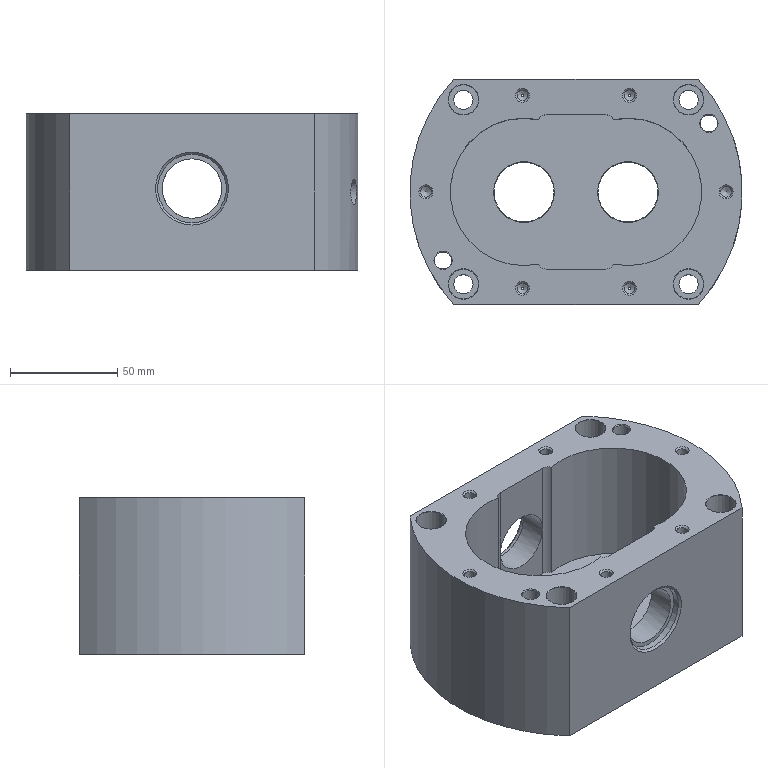NC program | NX | posted with a generic post | part box 155 x 105 x 73.2 mm
Lines 466 to 1316 of 30727:
(FLOOR_WALL_1_1 , TOOL : D25R0.5)
N912 T05 M6
N914 G54
N916 G17 G0 G90 X7.943 Y5.142 B0. C0. S2000 M3
N918 G43 Z30. H5
N920 Z1.5
N922 G94 G1 X6.744 Y5.554 Z1.467 F1000.
N924 X6.026 Y5.85 Z1.446
N926 X-6.026 Z1.131
N928 X-6.744 Y5.554 Z1.111
N930 X-8.656 Y4.897 Z1.058
N932 X-10.608 Y4.369 Z1.005
N934 X-12.591 Y3.974 Z0.952
N936 X-14.595 Y3.711 Z0.899
N938 X-16.613 Y3.584 Z0.846
N940 X-18.635 Y3.593 Z0.793
N942 X-20.652 Y3.736 Z0.74
N944 X-22.655 Y4.015 Z0.687
N946 X-23.416 Y4.167 Z0.667
N948 X-23.702 Y4.225 Z0.659
N950 X-24.464 Y4.255 Z0.639
N952 X-25.219 Y4.148 Z0.619
N954 X-25.943 Y3.909 Z0.599
N956 X-26.613 Y3.545 Z0.579
N958 X-27.207 Y3.067 Z0.559
N960 X-27.706 Y2.491 Z0.539
N962 X-28.095 Y1.835 Z0.519
N964 X-28.36 Y1.12 Z0.499
N966 X-28.475 Y0.548 Z0.484
N968 X-28.505 Y-0.214 Z0.464
N970 X-28.398 Y-0.969 Z0.444
N972 X-28.159 Y-1.693 Z0.424
N974 X-27.795 Y-2.363 Z0.404
N976 X-27.317 Y-2.957 Z0.384
N978 X-26.741 Y-3.456 Z0.364
N980 X-26.085 Y-3.845 Z0.344
N982 X-25.37 Y-4.11 Z0.324
N984 X-25.084 Y-4.167 Z0.317
N986 X-24.798 Y-4.225 Z0.309
N988 X-24.25 Y-4.26 Z0.295
N990 X-23.702 Y-4.225 Z0.28
N992 X-22.655 Y-4.015 Z0.252
N994 X-20.652 Y-3.736 Z0.199
N996 X-18.635 Y-3.593 Z0.146
N998 X-16.613 Y-3.584 Z0.093
N1000 X-14.595 Y-3.711 Z0.04
N1002 X-12.591 Y-3.974 Z-0.012
N1004 X-10.608 Y-4.369 Z-0.065
N1006 X-8.656 Y-4.897 Z-0.118
N1008 X-6.744 Y-5.554 Z-0.171
N1010 X-6.026 Y-5.85 Z-0.192
N1012 X0. Z-0.349
N1014 X6.026 F2200.
N1016 G2 X23.416 Y-4.167 R30.15
N1018 G3 X23.416 Y4.167 R-4.25
N1020 G2 X6.026 Y5.85 R30.15
N1022 G1 X-6.026
N1024 G2 X-23.416 Y4.167 R30.15
N1026 G3 X-23.416 Y-4.167 R-4.25
N1028 G2 X-6.026 Y-5.85 R30.15
N1030 G1 X0.
N1032 Y-23.35
N1034 X10.271
N1036 G2 X19.982 Y-21.327 R12.65
N1038 G3 X19.982 Y21.327 R-21.75
N1040 G2 X10.271 Y23.35 R12.65
N1042 G1 X-10.271
N1044 G2 X-19.982 Y21.327 R12.65
N1046 G3 X-19.982 Y-21.327 R-21.75
N1048 G2 X-10.271 Y-23.35 R12.65
N1050 G1 X0.
N1052 Z1.151
N1054 G0 X7.943 Y5.142
N1056 G1 X6.744 Y5.554 Z1.117 F1000.
N1058 X6.026 Y5.85 Z1.097
N1060 X-6.026 Z0.781
N1062 X-6.744 Y5.554 Z0.761
N1064 X-8.656 Y4.897 Z0.708
N1066 X-10.608 Y4.369 Z0.655
N1068 X-12.591 Y3.974 Z0.602
N1070 X-14.595 Y3.711 Z0.549
N1072 X-16.613 Y3.584 Z0.496
N1074 X-18.635 Y3.593 Z0.443
N1076 X-20.652 Y3.736 Z0.39
N1078 X-22.655 Y4.015 Z0.338
N1080 X-23.416 Y4.167 Z0.317
N1082 X-23.702 Y4.225 Z0.31
N1084 X-24.464 Y4.255 Z0.29
N1086 X-25.219 Y4.148 Z0.27
N1088 X-25.943 Y3.909 Z0.25
N1090 X-26.613 Y3.545 Z0.23
N1092 X-27.207 Y3.067 Z0.21
N1094 X-27.706 Y2.491 Z0.19
N1096 X-28.095 Y1.835 Z0.17
N1098 X-28.36 Y1.12 Z0.15
N1100 X-28.475 Y0.548 Z0.135
N1102 X-28.505 Y-0.214 Z0.115
N1104 X-28.398 Y-0.969 Z0.095
N1106 X-28.159 Y-1.693 Z0.075
N1108 X-27.795 Y-2.363 Z0.055
N1110 X-27.317 Y-2.957 Z0.035
N1112 X-26.741 Y-3.456 Z0.015
N1114 X-26.085 Y-3.845 Z-0.005
N1116 X-25.37 Y-4.11 Z-0.025
N1118 X-25.084 Y-4.167 Z-0.033
N1120 X-24.798 Y-4.225 Z-0.04
N1122 X-24.25 Y-4.26 Z-0.055
N1124 X-23.702 Y-4.225 Z-0.069
N1126 X-22.655 Y-4.015 Z-0.097
N1128 X-20.652 Y-3.736 Z-0.15
N1130 X-18.635 Y-3.593 Z-0.203
N1132 X-16.613 Y-3.584 Z-0.256
N1134 X-14.595 Y-3.711 Z-0.309
N1136 X-12.591 Y-3.974 Z-0.362
N1138 X-10.608 Y-4.369 Z-0.415
N1140 X-8.656 Y-4.897 Z-0.468
N1142 X-6.744 Y-5.554 Z-0.521
N1144 X-6.026 Y-5.85 Z-0.541
N1146 X0. Z-0.699
N1148 X6.026 F2200.
N1150 G2 X23.416 Y-4.167 R30.15
N1152 G3 X23.416 Y4.167 R-4.25
N1154 G2 X6.026 Y5.85 R30.15
N1156 G1 X-6.026
N1158 G2 X-23.416 Y4.167 R30.15
N1160 G3 X-23.416 Y-4.167 R-4.25
N1162 G2 X-6.026 Y-5.85 R30.15
N1164 G1 X0.
N1166 Y-23.35
N1168 X10.271
N1170 G2 X19.982 Y-21.327 R12.65
N1172 G3 X19.982 Y21.327 R-21.75
N1174 G2 X10.271 Y23.35 R12.65
N1176 G1 X-10.271
N1178 G2 X-19.982 Y21.327 R12.65
N1180 G3 X-19.982 Y-21.327 R-21.75
N1182 G2 X-10.271 Y-23.35 R12.65
N1184 G1 X0.
N1186 Z0.801
N1188 G0 X7.943 Y5.142
N1190 G1 X6.744 Y5.554 Z0.768 F1000.
N1192 X6.026 Y5.85 Z0.748
N1194 X-6.026 Z0.432
N1196 X-6.744 Y5.554 Z0.412
N1198 X-8.656 Y4.897 Z0.359
N1200 X-10.608 Y4.369 Z0.306
N1202 X-12.591 Y3.974 Z0.253
N1204 X-14.595 Y3.711 Z0.2
N1206 X-16.613 Y3.584 Z0.147
N1208 X-18.635 Y3.593 Z0.094
N1210 X-20.652 Y3.736 Z0.041
N1212 X-22.655 Y4.015 Z-0.012
N1214 X-23.416 Y4.167 Z-0.032
N1216 X-23.702 Y4.225 Z-0.04
N1218 X-24.464 Y4.255 Z-0.06
N1220 X-25.219 Y4.148 Z-0.08
N1222 X-25.943 Y3.909 Z-0.1
N1224 X-26.613 Y3.545 Z-0.12
N1226 X-27.207 Y3.067 Z-0.14
N1228 X-27.706 Y2.491 Z-0.16
N1230 X-28.095 Y1.835 Z-0.18
N1232 X-28.36 Y1.12 Z-0.2
N1234 X-28.475 Y0.548 Z-0.215
N1236 X-28.505 Y-0.214 Z-0.235
N1238 X-28.398 Y-0.969 Z-0.255
N1240 X-28.159 Y-1.693 Z-0.275
N1242 X-27.795 Y-2.363 Z-0.295
N1244 X-27.317 Y-2.957 Z-0.315
N1246 X-26.741 Y-3.456 Z-0.335
N1248 X-26.085 Y-3.845 Z-0.355
N1250 X-25.37 Y-4.11 Z-0.375
N1252 X-25.084 Y-4.167 Z-0.382
N1254 X-24.798 Y-4.225 Z-0.39
N1256 X-24.25 Y-4.26 Z-0.404
N1258 X-23.702 Y-4.225 Z-0.419
N1260 X-22.655 Y-4.015 Z-0.447
N1262 X-20.652 Y-3.736 Z-0.5
N1264 X-18.635 Y-3.593 Z-0.552
N1266 X-16.613 Y-3.584 Z-0.605
N1268 X-14.595 Y-3.711 Z-0.658
N1270 X-12.591 Y-3.974 Z-0.711
N1272 X-10.608 Y-4.369 Z-0.764
N1274 X-8.656 Y-4.897 Z-0.817
N1276 X-6.744 Y-5.554 Z-0.87
N1278 X-6.026 Y-5.85 Z-0.89
N1280 X0. Z-1.048
N1282 X6.026 F2200.
N1284 G2 X23.416 Y-4.167 R30.15
N1286 G3 X23.416 Y4.167 R-4.25
N1288 G2 X6.026 Y5.85 R30.15
N1290 G1 X-6.026
N1292 G2 X-23.416 Y4.167 R30.15
N1294 G3 X-23.416 Y-4.167 R-4.25
N1296 G2 X-6.026 Y-5.85 R30.15
N1298 G1 X0.
N1300 Y-23.35
N1302 X10.271
N1304 G2 X19.982 Y-21.327 R12.65
N1306 G3 X19.982 Y21.327 R-21.75
N1308 G2 X10.271 Y23.35 R12.65
N1310 G1 X-10.271
N1312 G2 X-19.982 Y21.327 R12.65
N1314 G3 X-19.982 Y-21.327 R-21.75
N1316 G2 X-10.271 Y-23.35 R12.65
N1318 G1 X0.
N1320 Z0.452
N1322 G0 X7.943 Y5.142
N1324 G1 X6.744 Y5.554 Z0.419 F1000.
N1326 X6.026 Y5.85 Z0.398
N1328 X-6.026 Z0.083
N1330 X-6.744 Y5.554 Z0.062
N1332 X-8.656 Y4.897 Z0.009
N1334 X-10.608 Y4.369 Z-0.044
N1336 X-12.591 Y3.974 Z-0.097
N1338 X-14.595 Y3.711 Z-0.15
N1340 X-16.613 Y3.584 Z-0.202
N1342 X-18.635 Y3.593 Z-0.255
N1344 X-20.652 Y3.736 Z-0.308
N1346 X-22.655 Y4.015 Z-0.361
N1348 X-23.416 Y4.167 Z-0.382
N1350 X-23.702 Y4.225 Z-0.389
N1352 X-24.464 Y4.255 Z-0.409
N1354 X-25.219 Y4.148 Z-0.429
N1356 X-25.943 Y3.909 Z-0.449
N1358 X-26.613 Y3.545 Z-0.469
N1360 X-27.207 Y3.067 Z-0.489
N1362 X-27.706 Y2.491 Z-0.509
N1364 X-28.095 Y1.835 Z-0.529
N1366 X-28.36 Y1.12 Z-0.549
N1368 X-28.475 Y0.548 Z-0.564
N1370 X-28.505 Y-0.214 Z-0.584
N1372 X-28.398 Y-0.969 Z-0.604
N1374 X-28.159 Y-1.693 Z-0.624
N1376 X-27.795 Y-2.363 Z-0.644
N1378 X-27.317 Y-2.957 Z-0.664
N1380 X-26.741 Y-3.456 Z-0.684
N1382 X-26.085 Y-3.845 Z-0.704
N1384 X-25.37 Y-4.11 Z-0.724
N1386 X-25.084 Y-4.167 Z-0.732
N1388 X-24.798 Y-4.225 Z-0.739
N1390 X-24.25 Y-4.26 Z-0.754
N1392 X-23.702 Y-4.225 Z-0.768
N1394 X-22.655 Y-4.015 Z-0.796
N1396 X-20.652 Y-3.736 Z-0.849
N1398 X-18.635 Y-3.593 Z-0.902
N1400 X-16.613 Y-3.584 Z-0.955
N1402 X-14.595 Y-3.711 Z-1.008
N1404 X-12.591 Y-3.974 Z-1.061
N1406 X-10.608 Y-4.369 Z-1.114
N1408 X-8.656 Y-4.897 Z-1.167
N1410 X-6.744 Y-5.554 Z-1.22
N1412 X-6.026 Y-5.85 Z-1.24
N1414 X0. Z-1.398
N1416 X6.026 F2200.
N1418 G2 X23.416 Y-4.167 R30.15
N1420 G3 X23.416 Y4.167 R-4.25
N1422 G2 X6.026 Y5.85 R30.15
N1424 G1 X-6.026
N1426 G2 X-23.416 Y4.167 R30.15
N1428 G3 X-23.416 Y-4.167 R-4.25
N1430 G2 X-6.026 Y-5.85 R30.15
N1432 G1 X0.
N1434 Y-23.35
N1436 X10.271
N1438 G2 X19.982 Y-21.327 R12.65
N1440 G3 X19.982 Y21.327 R-21.75
N1442 G2 X10.271 Y23.35 R12.65
N1444 G1 X-10.271
N1446 G2 X-19.982 Y21.327 R12.65
N1448 G3 X-19.982 Y-21.327 R-21.75
N1450 G2 X-10.271 Y-23.35 R12.65
N1452 G1 X0.
N1454 Z0.102
N1456 G0 X7.943 Y5.142
N1458 G1 X6.744 Y5.554 Z0.069 F1000.
N1460 X6.026 Y5.85 Z0.049
N1462 X-6.026 Z-0.267
N1464 X-6.744 Y5.554 Z-0.287
N1466 X-8.656 Y4.897 Z-0.34
N1468 X-10.608 Y4.369 Z-0.393
N1470 X-12.591 Y3.974 Z-0.446
N1472 X-14.595 Y3.711 Z-0.499
N1474 X-16.613 Y3.584 Z-0.552
N1476 X-18.635 Y3.593 Z-0.605
N1478 X-20.652 Y3.736 Z-0.658
N1480 X-22.655 Y4.015 Z-0.711
N1482 X-23.416 Y4.167 Z-0.731
N1484 X-23.702 Y4.225 Z-0.739
N1486 X-24.464 Y4.255 Z-0.759
N1488 X-25.219 Y4.148 Z-0.779
N1490 X-25.943 Y3.909 Z-0.799
N1492 X-26.613 Y3.545 Z-0.819
N1494 X-27.207 Y3.067 Z-0.839
N1496 X-27.706 Y2.491 Z-0.858
N1498 X-28.095 Y1.835 Z-0.878
N1500 X-28.36 Y1.12 Z-0.898
N1502 X-28.475 Y0.548 Z-0.914
N1504 X-28.505 Y-0.214 Z-0.934
N1506 X-28.398 Y-0.969 Z-0.954
N1508 X-28.159 Y-1.693 Z-0.974
N1510 X-27.795 Y-2.363 Z-0.994
N1512 X-27.317 Y-2.957 Z-1.014
N1514 X-26.741 Y-3.456 Z-1.033
N1516 X-26.085 Y-3.845 Z-1.053
N1518 X-25.37 Y-4.11 Z-1.073
N1520 X-25.084 Y-4.167 Z-1.081
N1522 X-24.798 Y-4.225 Z-1.089
N1524 X-24.25 Y-4.26 Z-1.103
N1526 X-23.702 Y-4.225 Z-1.117
N1528 X-22.655 Y-4.015 Z-1.145
N1530 X-20.652 Y-3.736 Z-1.198
N1532 X-18.635 Y-3.593 Z-1.251
N1534 X-16.613 Y-3.584 Z-1.304
N1536 X-14.595 Y-3.711 Z-1.357
N1538 X-12.591 Y-3.974 Z-1.41
N1540 X-10.608 Y-4.369 Z-1.463
N1542 X-8.656 Y-4.897 Z-1.516
N1544 X-6.744 Y-5.554 Z-1.569
N1546 X-6.026 Y-5.85 Z-1.589
N1548 X0. Z-1.747
N1550 X6.026 F2200.
N1552 G2 X23.416 Y-4.167 R30.15
N1554 G3 X23.416 Y4.167 R-4.25
N1556 G2 X6.026 Y5.85 R30.15
N1558 G1 X-6.026
N1560 G2 X-23.416 Y4.167 R30.15
N1562 G3 X-23.416 Y-4.167 R-4.25
N1564 G2 X-6.026 Y-5.85 R30.15
N1566 G1 X0.
N1568 Y-23.35
N1570 X10.271
N1572 G2 X19.982 Y-21.327 R12.65
N1574 G3 X19.982 Y21.327 R-21.75
N1576 G2 X10.271 Y23.35 R12.65
N1578 G1 X-10.271
N1580 G2 X-19.982 Y21.327 R12.65
N1582 G3 X-19.982 Y-21.327 R-21.75
N1584 G2 X-10.271 Y-23.35 R12.65
N1586 G1 X0.
N1588 Z-0.247
N1590 G0 X7.943 Y5.142
N1592 G1 X6.744 Y5.554 Z-0.28 F1000.
N1594 X6.026 Y5.85 Z-0.301
N1596 X-6.026 Z-0.616
N1598 X-6.744 Y5.554 Z-0.637
N1600 X-8.656 Y4.897 Z-0.69
N1602 X-10.608 Y4.369 Z-0.742
N1604 X-12.591 Y3.974 Z-0.795
N1606 X-14.595 Y3.711 Z-0.848
N1608 X-16.613 Y3.584 Z-0.901
N1610 X-18.635 Y3.593 Z-0.954
N1612 X-20.652 Y3.736 Z-1.007
N1614 X-22.655 Y4.015 Z-1.06
N1616 X-23.416 Y4.167 Z-1.08
N1618 X-23.702 Y4.225 Z-1.088
N1620 X-24.464 Y4.255 Z-1.108
N1622 X-25.219 Y4.148 Z-1.128
N1624 X-25.943 Y3.909 Z-1.148
N1626 X-26.613 Y3.545 Z-1.168
N1628 X-27.207 Y3.067 Z-1.188
N1630 X-27.706 Y2.491 Z-1.208
N1632 X-28.095 Y1.835 Z-1.228
N1634 X-28.36 Y1.12 Z-1.248
N1636 X-28.475 Y0.548 Z-1.263
N1638 X-28.505 Y-0.214 Z-1.283
N1640 X-28.398 Y-0.969 Z-1.303
N1642 X-28.159 Y-1.693 Z-1.323
N1644 X-27.795 Y-2.363 Z-1.343
N1646 X-27.317 Y-2.957 Z-1.363
N1648 X-26.741 Y-3.456 Z-1.383
N1650 X-26.085 Y-3.845 Z-1.403
N1652 X-25.37 Y-4.11 Z-1.423
N1654 X-25.084 Y-4.167 Z-1.43
N1656 X-24.798 Y-4.225 Z-1.438
N1658 X-24.25 Y-4.26 Z-1.452
N1660 X-23.702 Y-4.225 Z-1.467
N1662 X-22.655 Y-4.015 Z-1.495
N1664 X-20.652 Y-3.736 Z-1.548
N1666 X-18.635 Y-3.593 Z-1.601
N1668 X-16.613 Y-3.584 Z-1.654
N1670 X-14.595 Y-3.711 Z-1.707
N1672 X-12.591 Y-3.974 Z-1.76
N1674 X-10.608 Y-4.369 Z-1.812
N1676 X-8.656 Y-4.897 Z-1.865
N1678 X-6.744 Y-5.554 Z-1.918
N1680 X-6.026 Y-5.85 Z-1.939
N1682 X0. Z-2.097
N1684 X6.026 F2200.
N1686 G2 X23.416 Y-4.167 R30.15
N1688 G3 X23.416 Y4.167 R-4.25
N1690 G2 X6.026 Y5.85 R30.15
N1692 G1 X-6.026
N1694 G2 X-23.416 Y4.167 R30.15
N1696 G3 X-23.416 Y-4.167 R-4.25
N1698 G2 X-6.026 Y-5.85 R30.15
N1700 G1 X0.
N1702 Y-23.35
N1704 X10.271
N1706 G2 X19.982 Y-21.327 R12.65
N1708 G3 X19.982 Y21.327 R-21.75
N1710 G2 X10.271 Y23.35 R12.65
N1712 G1 X-10.271
N1714 G2 X-19.982 Y21.327 R12.65
N1716 G3 X-19.982 Y-21.327 R-21.75
N1718 G2 X-10.271 Y-23.35 R12.65
N1720 G1 X0.
N1722 Z-0.597
N1724 G0 X7.943 Y5.142
N1726 G1 X6.744 Y5.554 Z-0.63 F1000.
N1728 X6.026 Y5.85 Z-0.65
N1730 X-6.026 Z-0.966
N1732 X-6.744 Y5.554 Z-0.986
N1734 X-8.656 Y4.897 Z-1.039
N1736 X-10.608 Y4.369 Z-1.092
N1738 X-12.591 Y3.974 Z-1.145
N1740 X-14.595 Y3.711 Z-1.198
N1742 X-16.613 Y3.584 Z-1.251
N1744 X-18.635 Y3.593 Z-1.304
N1746 X-20.652 Y3.736 Z-1.357
N1748 X-22.655 Y4.015 Z-1.41
N1750 X-23.416 Y4.167 Z-1.43
N1752 X-23.702 Y4.225 Z-1.438
N1754 X-24.464 Y4.255 Z-1.457
N1756 X-25.219 Y4.148 Z-1.477
N1758 X-25.943 Y3.909 Z-1.497
N1760 X-26.613 Y3.545 Z-1.517
N1762 X-27.207 Y3.067 Z-1.537
N1764 X-27.706 Y2.491 Z-1.557
N1766 X-28.095 Y1.835 Z-1.577
N1768 X-28.36 Y1.12 Z-1.597
N1770 X-28.475 Y0.548 Z-1.613
N1772 X-28.505 Y-0.214 Z-1.632
N1774 X-28.398 Y-0.969 Z-1.652
N1776 X-28.159 Y-1.693 Z-1.672
N1778 X-27.795 Y-2.363 Z-1.692
N1780 X-27.317 Y-2.957 Z-1.712
N1782 X-26.741 Y-3.456 Z-1.732
N1784 X-26.085 Y-3.845 Z-1.752
N1786 X-25.37 Y-4.11 Z-1.772
N1788 X-25.084 Y-4.167 Z-1.78
N1790 X-24.798 Y-4.225 Z-1.788
N1792 X-24.25 Y-4.26 Z-1.802
N1794 X-23.702 Y-4.225 Z-1.816
N1796 X-22.655 Y-4.015 Z-1.844
N1798 X-20.652 Y-3.736 Z-1.897
N1800 X-18.635 Y-3.593 Z-1.95
N1802 X-16.613 Y-3.584 Z-2.003
N1804 X-14.595 Y-3.711 Z-2.056
N1806 X-12.591 Y-3.974 Z-2.109
N1808 X-10.608 Y-4.369 Z-2.162
N1810 X-8.656 Y-4.897 Z-2.215
N1812 X-6.744 Y-5.554 Z-2.268
N1814 X-6.026 Y-5.85 Z-2.288
N1816 X0. Z-2.446
N1818 X6.026 F2200.
N1820 G2 X23.416 Y-4.167 R30.15
N1822 G3 X23.416 Y4.167 R-4.25
N1824 G2 X6.026 Y5.85 R30.15
N1826 G1 X-6.026
N1828 G2 X-23.416 Y4.167 R30.15
N1830 G3 X-23.416 Y-4.167 R-4.25
N1832 G2 X-6.026 Y-5.85 R30.15
N1834 G1 X0.
N1836 Y-23.35
N1838 X10.271
N1840 G2 X19.982 Y-21.327 R12.65
N1842 G3 X19.982 Y21.327 R-21.75
N1844 G2 X10.271 Y23.35 R12.65
N1846 G1 X-10.271
N1848 G2 X-19.982 Y21.327 R12.65
N1850 G3 X-19.982 Y-21.327 R-21.75
N1852 G2 X-10.271 Y-23.35 R12.65
N1854 G1 X0.
N1856 Z-0.946
N1858 G0 X7.943 Y5.142
N1860 G1 X6.744 Y5.554 Z-0.979 F1000.
N1862 X6.026 Y5.85 Z-0.999
N1864 X-6.026 Z-1.315
N1866 X-6.744 Y5.554 Z-1.335
N1868 X-8.656 Y4.897 Z-1.388
N1870 X-10.608 Y4.369 Z-1.441
N1872 X-12.591 Y3.974 Z-1.494
N1874 X-14.595 Y3.711 Z-1.547
N1876 X-16.613 Y3.584 Z-1.6
N1878 X-18.635 Y3.593 Z-1.653
N1880 X-20.652 Y3.736 Z-1.706
N1882 X-22.655 Y4.015 Z-1.759
N1884 X-23.416 Y4.167 Z-1.779
N1886 X-23.702 Y4.225 Z-1.787
N1888 X-24.464 Y4.255 Z-1.807
N1890 X-25.219 Y4.148 Z-1.827
N1892 X-25.943 Y3.909 Z-1.847
N1894 X-26.613 Y3.545 Z-1.867
N1896 X-27.207 Y3.067 Z-1.887
N1898 X-27.706 Y2.491 Z-1.907
N1900 X-28.095 Y1.835 Z-1.927
N1902 X-28.36 Y1.12 Z-1.947
N1904 X-28.475 Y0.548 Z-1.962
N1906 X-28.505 Y-0.214 Z-1.982
N1908 X-28.398 Y-0.969 Z-2.002
N1910 X-28.159 Y-1.693 Z-2.022
N1912 X-27.795 Y-2.363 Z-2.042
N1914 X-27.317 Y-2.957 Z-2.062
N1916 X-26.741 Y-3.456 Z-2.082
N1918 X-26.085 Y-3.845 Z-2.102
N1920 X-25.37 Y-4.11 Z-2.122
N1922 X-25.084 Y-4.167 Z-2.129
N1924 X-24.798 Y-4.225 Z-2.137
N1926 X-24.25 Y-4.26 Z-2.151
N1928 X-23.702 Y-4.225 Z-2.166
N1930 X-22.655 Y-4.015 Z-2.194
N1932 X-20.652 Y-3.736 Z-2.247
N1934 X-18.635 Y-3.593 Z-2.3
N1936 X-16.613 Y-3.584 Z-2.352
N1938 X-14.595 Y-3.711 Z-2.405
N1940 X-12.591 Y-3.974 Z-2.458
N1942 X-10.608 Y-4.369 Z-2.511
N1944 X-8.656 Y-4.897 Z-2.564
N1946 X-6.744 Y-5.554 Z-2.617
N1948 X-6.026 Y-5.85 Z-2.638
N1950 X0. Z-2.795
N1952 X6.026 F2200.
N1954 G2 X23.416 Y-4.167 R30.15
N1956 G3 X23.416 Y4.167 R-4.25
N1958 G2 X6.026 Y5.85 R30.15
N1960 G1 X-6.026
N1962 G2 X-23.416 Y4.167 R30.15
N1964 G3 X-23.416 Y-4.167 R-4.25
N1966 G2 X-6.026 Y-5.85 R30.15
N1968 G1 X0.
N1970 Y-23.35
N1972 X10.271
N1974 G2 X19.982 Y-21.327 R12.65
N1976 G3 X19.982 Y21.327 R-21.75
N1978 G2 X10.271 Y23.35 R12.65
N1980 G1 X-10.271
N1982 G2 X-19.982 Y21.327 R12.65
N1984 G3 X-19.982 Y-21.327 R-21.75
N1986 G2 X-10.271 Y-23.35 R12.65
N1988 G1 X0.
N1990 Z-1.295
N1992 G0 X7.943 Y5.142
N1994 G1 X6.744 Y5.554 Z-1.329 F1000.
N1996 X6.026 Y5.85 Z-1.349
N1998 X-6.026 Z-1.664
N2000 X-6.744 Y5.554 Z-1.685
N2002 X-8.656 Y4.897 Z-1.738
N2004 X-10.608 Y4.369 Z-1.791
N2006 X-12.591 Y3.974 Z-1.844
N2008 X-14.595 Y3.711 Z-1.897
N2010 X-16.613 Y3.584 Z-1.95
N2012 X-18.635 Y3.593 Z-2.002
N2014 X-20.652 Y3.736 Z-2.055
N2016 X-22.655 Y4.015 Z-2.108
N2018 X-23.416 Y4.167 Z-2.129
N2020 X-23.702 Y4.225 Z-2.136
N2022 X-24.464 Y4.255 Z-2.156
N2024 X-25.219 Y4.148 Z-2.176
N2026 X-25.943 Y3.909 Z-2.196
N2028 X-26.613 Y3.545 Z-2.216
N2030 X-27.207 Y3.067 Z-2.236
N2032 X-27.706 Y2.491 Z-2.256
N2034 X-28.095 Y1.835 Z-2.276
N2036 X-28.36 Y1.12 Z-2.296
N2038 X-28.475 Y0.548 Z-2.311
N2040 X-28.505 Y-0.214 Z-2.331
N2042 X-28.398 Y-0.969 Z-2.351
N2044 X-28.159 Y-1.693 Z-2.371
N2046 X-27.795 Y-2.363 Z-2.391
N2048 X-27.317 Y-2.957 Z-2.411
N2050 X-26.741 Y-3.456 Z-2.431
N2052 X-26.085 Y-3.845 Z-2.451
N2054 X-25.37 Y-4.11 Z-2.471
N2056 X-25.084 Y-4.167 Z-2.479
N2058 X-24.798 Y-4.225 Z-2.486
N2060 X-24.25 Y-4.26 Z-2.501
N2062 X-23.702 Y-4.225 Z-2.515
N2064 X-22.655 Y-4.015 Z-2.543
N2066 X-20.652 Y-3.736 Z-2.596
N2068 X-18.635 Y-3.593 Z-2.649
N2070 X-16.613 Y-3.584 Z-2.702
N2072 X-14.595 Y-3.711 Z-2.755
N2074 X-12.591 Y-3.974 Z-2.808
N2076 X-10.608 Y-4.369 Z-2.861
N2078 X-8.656 Y-4.897 Z-2.914
N2080 X-6.744 Y-5.554 Z-2.967
N2082 X-6.026 Y-5.85 Z-2.987
N2084 X0. Z-3.145
N2086 X6.026 F2200.
N2088 G2 X23.416 Y-4.167 R30.15
N2090 G3 X23.416 Y4.167 R-4.25
N2092 G2 X6.026 Y5.85 R30.15
N2094 G1 X-6.026
N2096 G2 X-23.416 Y4.167 R30.15
N2098 G3 X-23.416 Y-4.167 R-4.25
N2100 G2 X-6.026 Y-5.85 R30.15
N2102 G1 X0.
N2104 Y-23.35
N2106 X10.271
N2108 G2 X19.982 Y-21.327 R12.65
N2110 G3 X19.982 Y21.327 R-21.75
N2112 G2 X10.271 Y23.35 R12.65
N2114 G1 X-10.271
N2116 G2 X-19.982 Y21.327 R12.65
N2118 G3 X-19.982 Y-21.327 R-21.75
N2120 G2 X-10.271 Y-23.35 R12.65
N2122 G1 X0.
N2124 Z-1.645
N2126 G0 X7.943 Y5.142
N2128 G1 X6.744 Y5.554 Z-1.678 F1000.
N2130 X6.026 Y5.85 Z-1.698
N2132 X-6.026 Z-2.014
N2134 X-6.744 Y5.554 Z-2.034
N2136 X-8.656 Y4.897 Z-2.087
N2138 X-10.608 Y4.369 Z-2.14
N2140 X-12.591 Y3.974 Z-2.193
N2142 X-14.595 Y3.711 Z-2.246
N2144 X-16.613 Y3.584 Z-2.299
N2146 X-18.635 Y3.593 Z-2.352
N2148 X-20.652 Y3.736 Z-2.405
N2150 X-22.655 Y4.015 Z-2.458
N2152 X-23.416 Y4.167 Z-2.478
N2154 X-23.702 Y4.225 Z-2.486
N2156 X-24.464 Y4.255 Z-2.506
N2158 X-25.219 Y4.148 Z-2.526
N2160 X-25.943 Y3.909 Z-2.546
N2162 X-26.613 Y3.545 Z-2.566
N2164 X-27.207 Y3.067 Z-2.586
N2166 X-27.706 Y2.491 Z-2.606
N2168 X-28.095 Y1.835 Z-2.626
N2170 X-28.36 Y1.12 Z-2.645
N2172 X-28.475 Y0.548 Z-2.661
N2174 X-28.505 Y-0.214 Z-2.681
N2176 X-28.398 Y-0.969 Z-2.701
N2178 X-28.159 Y-1.693 Z-2.721
N2180 X-27.795 Y-2.363 Z-2.741
N2182 X-27.317 Y-2.957 Z-2.761
N2184 X-26.741 Y-3.456 Z-2.781
N2186 X-26.085 Y-3.845 Z-2.801
N2188 X-25.37 Y-4.11 Z-2.82
N2190 X-25.084 Y-4.167 Z-2.828
N2192 X-24.798 Y-4.225 Z-2.836
N2194 X-24.25 Y-4.26 Z-2.85
N2196 X-23.702 Y-4.225 Z-2.865
N2198 X-22.655 Y-4.015 Z-2.892
N2200 X-20.652 Y-3.736 Z-2.945
N2202 X-18.635 Y-3.593 Z-2.998
N2204 X-16.613 Y-3.584 Z-3.051
N2206 X-14.595 Y-3.711 Z-3.104
N2208 X-12.591 Y-3.974 Z-3.157
N2210 X-10.608 Y-4.369 Z-3.21
N2212 X-8.656 Y-4.897 Z-3.263
N2214 X-6.744 Y-5.554 Z-3.316
N2216 X-6.026 Y-5.85 Z-3.336
N2218 X0. Z-3.494
N2220 X6.026 F2200.
N2222 G2 X23.416 Y-4.167 R30.15
N2224 G3 X23.416 Y4.167 R-4.25
N2226 G2 X6.026 Y5.85 R30.15
N2228 G1 X-6.026
N2230 G2 X-23.416 Y4.167 R30.15
N2232 G3 X-23.416 Y-4.167 R-4.25
N2234 G2 X-6.026 Y-5.85 R30.15
N2236 G1 X0.
N2238 Y-23.35
N2240 X10.271
N2242 G2 X19.982 Y-21.327 R12.65
N2244 G3 X19.982 Y21.327 R-21.75
N2246 G2 X10.271 Y23.35 R12.65
N2248 G1 X-10.271
N2250 G2 X-19.982 Y21.327 R12.65
N2252 G3 X-19.982 Y-21.327 R-21.75
N2254 G2 X-10.271 Y-23.35 R12.65
N2256 G1 X0.
N2258 Z-1.994
N2260 G0 X7.943 Y5.142
N2262 G1 X6.744 Y5.554 Z-2.027 F1000.
N2264 X6.026 Y5.85 Z-2.048
N2266 X-6.026 Z-2.363
N2268 X-6.744 Y5.554 Z-2.384
N2270 X-8.656 Y4.897 Z-2.437
N2272 X-10.608 Y4.369 Z-2.49
N2274 X-12.591 Y3.974 Z-2.542
N2276 X-14.595 Y3.711 Z-2.595
N2278 X-16.613 Y3.584 Z-2.648
N2280 X-18.635 Y3.593 Z-2.701
N2282 X-20.652 Y3.736 Z-2.754
N2284 X-22.655 Y4.015 Z-2.807
N2286 X-23.416 Y4.167 Z-2.828
N2288 X-23.702 Y4.225 Z-2.835
N2290 X-24.464 Y4.255 Z-2.855
N2292 X-25.219 Y4.148 Z-2.875
N2294 X-25.943 Y3.909 Z-2.895
N2296 X-26.613 Y3.545 Z-2.915
N2298 X-27.207 Y3.067 Z-2.935
N2300 X-27.706 Y2.491 Z-2.955
N2302 X-28.095 Y1.835 Z-2.975
N2304 X-28.36 Y1.12 Z-2.995
N2306 X-28.475 Y0.548 Z-3.01
N2308 X-28.505 Y-0.214 Z-3.03
N2310 X-28.398 Y-0.969 Z-3.05
N2312 X-28.159 Y-1.693 Z-3.07
N2314 X-27.795 Y-2.363 Z-3.09
N2316 X-27.317 Y-2.957 Z-3.11
N2318 X-26.741 Y-3.456 Z-3.13
N2320 X-26.085 Y-3.845 Z-3.15
N2322 X-25.37 Y-4.11 Z-3.17
N2324 X-25.084 Y-4.167 Z-3.178
N2326 X-24.798 Y-4.225 Z-3.185
N2328 X-24.25 Y-4.26 Z-3.2
N2330 X-23.702 Y-4.225 Z-3.214
N2332 X-22.655 Y-4.015 Z-3.242
N2334 X-20.652 Y-3.736 Z-3.295
N2336 X-18.635 Y-3.593 Z-3.348
N2338 X-16.613 Y-3.584 Z-3.401
N2340 X-14.595 Y-3.711 Z-3.454
N2342 X-12.591 Y-3.974 Z-3.507
N2344 X-10.608 Y-4.369 Z-3.56
N2346 X-8.656 Y-4.897 Z-3.613
N2348 X-6.744 Y-5.554 Z-3.665
N2350 X-6.026 Y-5.85 Z-3.686
N2352 X0. Z-3.844
N2354 X6.026 F2200.
N2356 G2 X23.416 Y-4.167 R30.15
N2358 G3 X23.416 Y4.167 R-4.25
N2360 G2 X6.026 Y5.85 R30.15
N2362 G1 X-6.026
N2364 G2 X-23.416 Y4.167 R30.15
N2366 G3 X-23.416 Y-4.167 R-4.25
N2368 G2 X-6.026 Y-5.85 R30.15
N2370 G1 X0.
N2372 Y-23.35
N2374 X10.271
N2376 G2 X19.982 Y-21.327 R12.65
N2378 G3 X19.982 Y21.327 R-21.75
N2380 G2 X10.271 Y23.35 R12.65
N2382 G1 X-10.271
N2384 G2 X-19.982 Y21.327 R12.65
N2386 G3 X-19.982 Y-21.327 R-21.75
N2388 G2 X-10.271 Y-23.35 R12.65
N2390 G1 X0.
N2392 Z-2.344
N2394 G0 X7.943 Y5.142
N2396 G1 X6.744 Y5.554 Z-2.377 F1000.
N2398 X6.026 Y5.85 Z-2.397
N2400 X-6.026 Z-2.713
N2402 X-6.744 Y5.554 Z-2.733
N2404 X-8.656 Y4.897 Z-2.786
N2406 X-10.608 Y4.369 Z-2.839
N2408 X-12.591 Y3.974 Z-2.892
N2410 X-14.595 Y3.711 Z-2.945
N2412 X-16.613 Y3.584 Z-2.998
N2414 X-18.635 Y3.593 Z-3.051
N2416 X-20.652 Y3.736 Z-3.104
N2418 X-22.655 Y4.015 Z-3.157
N2420 X-23.416 Y4.167 Z-3.177
N2422 X-23.702 Y4.225 Z-3.185
N2424 X-24.464 Y4.255 Z-3.205
N2426 X-25.219 Y4.148 Z-3.225
N2428 X-25.943 Y3.909 Z-3.245
N2430 X-26.613 Y3.545 Z-3.264
N2432 X-27.207 Y3.067 Z-3.284
N2434 X-27.706 Y2.491 Z-3.304
N2436 X-28.095 Y1.835 Z-3.324
N2438 X-28.36 Y1.12 Z-3.344
N2440 X-28.475 Y0.548 Z-3.36
N2442 X-28.505 Y-0.214 Z-3.38
N2444 X-28.398 Y-0.969 Z-3.4
N2446 X-28.159 Y-1.693 Z-3.42
N2448 X-27.795 Y-2.363 Z-3.439
N2450 X-27.317 Y-2.957 Z-3.459
N2452 X-26.741 Y-3.456 Z-3.479
N2454 X-26.085 Y-3.845 Z-3.499
N2456 X-25.37 Y-4.11 Z-3.519
N2458 X-25.084 Y-4.167 Z-3.527
N2460 X-24.798 Y-4.225 Z-3.535
N2462 X-24.25 Y-4.26 Z-3.549
N2464 X-23.702 Y-4.225 Z-3.563
N2466 X-22.655 Y-4.015 Z-3.591
N2468 X-20.652 Y-3.736 Z-3.644
N2470 X-18.635 Y-3.593 Z-3.697
N2472 X-16.613 Y-3.584 Z-3.75
N2474 X-14.595 Y-3.711 Z-3.803
N2476 X-12.591 Y-3.974 Z-3.856
N2478 X-10.608 Y-4.369 Z-3.909
N2480 X-8.656 Y-4.897 Z-3.962
N2482 X-6.744 Y-5.554 Z-4.015
N2484 X-6.026 Y-5.85 Z-4.035
N2486 X0. Z-4.193
N2488 X6.026 F2200.
N2490 G2 X23.416 Y-4.167 R30.15
N2492 G3 X23.416 Y4.167 R-4.25
N2494 G2 X6.026 Y5.85 R30.15
N2496 G1 X-6.026
N2498 G2 X-23.416 Y4.167 R30.15
N2500 G3 X-23.416 Y-4.167 R-4.25
N2502 G2 X-6.026 Y-5.85 R30.15
N2504 G1 X0.
N2506 Y-23.35
N2508 X10.271
N2510 G2 X19.982 Y-21.327 R12.65
N2512 G3 X19.982 Y21.327 R-21.75
N2514 G2 X10.271 Y23.35 R12.65
N2516 G1 X-10.271
N2518 G2 X-19.982 Y21.327 R12.65
N2520 G3 X-19.982 Y-21.327 R-21.75
N2522 G2 X-10.271 Y-23.35 R12.65
N2524 G1 X0.
N2526 Z-2.693
N2528 G0 X7.943 Y5.142
N2530 G1 X6.744 Y5.554 Z-2.726 F1000.
N2532 X6.026 Y5.85 Z-2.747
N2534 X-6.026 Z-3.062
N2536 X-6.744 Y5.554 Z-3.082
N2538 X-8.656 Y4.897 Z-3.135
N2540 X-10.608 Y4.369 Z-3.188
N2542 X-12.591 Y3.974 Z-3.241
N2544 X-14.595 Y3.711 Z-3.294
N2546 X-16.613 Y3.584 Z-3.347
N2548 X-18.635 Y3.593 Z-3.4
N2550 X-20.652 Y3.736 Z-3.453
N2552 X-22.655 Y4.015 Z-3.506
N2554 X-23.416 Y4.167 Z-3.526
N2556 X-23.702 Y4.225 Z-3.534
N2558 X-24.464 Y4.255 Z-3.554
N2560 X-25.219 Y4.148 Z-3.574
N2562 X-25.943 Y3.909 Z-3.594
N2564 X-26.613 Y3.545 Z-3.614
N2566 X-27.207 Y3.067 Z-3.634
N2568 X-27.706 Y2.491 Z-3.654
N2570 X-28.095 Y1.835 Z-3.674
N2572 X-28.36 Y1.12 Z-3.694
N2574 X-28.475 Y0.548 Z-3.709
N2576 X-28.505 Y-0.214 Z-3.729
N2578 X-28.398 Y-0.969 Z-3.749
N2580 X-28.159 Y-1.693 Z-3.769
N2582 X-27.795 Y-2.363 Z-3.789
N2584 X-27.317 Y-2.957 Z-3.809
N2586 X-26.741 Y-3.456 Z-3.829
N2588 X-26.085 Y-3.845 Z-3.849
N2590 X-25.37 Y-4.11 Z-3.869
N2592 X-25.084 Y-4.167 Z-3.876
N2594 X-24.798 Y-4.225 Z-3.884
N2596 X-24.25 Y-4.26 Z-3.898
N2598 X-23.702 Y-4.225 Z-3.913
N2600 X-22.655 Y-4.015 Z-3.941
N2602 X-20.652 Y-3.736 Z-3.994
N2604 X-18.635 Y-3.593 Z-4.047
N2606 X-16.613 Y-3.584 Z-4.1